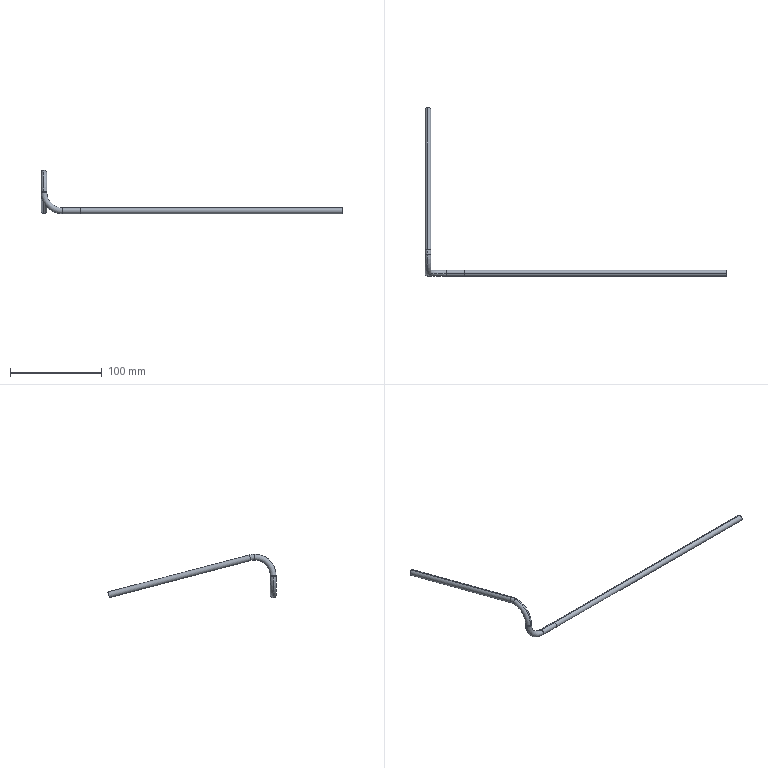Part | STEP file | copper tube 33_default_machined_ | 2 solids | 20 faces | box 328.675 x 183.099 x 47.35 mm | volume 11843 mm3 | cylinder 10 | torus 6 | plane 4 | commonest cylinder face diameters 6.35 x8 4.75 x2
STEP:
#1=CARTESIAN_POINT('',(0.,0.,0.));
#2=DIRECTION('',(0.,0.,1.));
#3=DIRECTION('',(1.,0.,0.));
#4=AXIS2_PLACEMENT_3D('',#1,#2,#3);
#5=CARTESIAN_POINT('',(285.5,0.,3.175));
#6=VERTEX_POINT('',#5);
#7=CARTESIAN_POINT('',(285.5,0.,-3.175));
#8=VERTEX_POINT('',#7);
#9=CARTESIAN_POINT('',(285.5,0.,0.));
#10=DIRECTION('',(-1.,0.,0.));
#11=DIRECTION('',(0.,0.,1.));
#12=AXIS2_PLACEMENT_3D('',#9,#10,#11);
#13=CIRCLE('',#12,3.175);
#14=CARTESIAN_POINT('',(285.5,0.,0.));
#15=DIRECTION('',(-1.,0.,0.));
#16=DIRECTION('',(0.,0.,1.));
#17=AXIS2_PLACEMENT_3D('',#14,#15,#16);
#18=CYLINDRICAL_SURFACE('',#17,3.175);
#19=CARTESIAN_POINT('',(0.,0.));
#20=DIRECTION('',(1.,0.));
#21=VECTOR('',#20,1.);
#22=LINE('',#19,#21);
#23=(GEOMETRIC_REPRESENTATION_CONTEXT(2)PARAMETRIC_REPRESENTATION_CONTEXT()REPRESENTATION_CONTEXT('',''));
#24=DEFINITIONAL_REPRESENTATION('',(#22),#23);
#25=PCURVE('',#18,#24);
#26=CARTESIAN_POINT('',(285.5,0.,0.));
#27=DIRECTION('',(1.,0.,0.));
#28=DIRECTION('',(0.,0.,-1.));
#29=AXIS2_PLACEMENT_3D('',#26,#27,#28);
#30=PLANE('',#29);
#31=CARTESIAN_POINT('',(-3.175,0.));
#32=CARTESIAN_POINT('',(-3.175,5.499));
#33=CARTESIAN_POINT('',(1.587,2.75));
#34=CARTESIAN_POINT('',(6.35,0.));
#35=CARTESIAN_POINT('',(1.587,-2.75));
#36=CARTESIAN_POINT('',(-3.175,-5.499));
#37=CARTESIAN_POINT('',(-3.175,0.));
#38=(BOUNDED_CURVE()B_SPLINE_CURVE(2,(#31,#32,#33,#34,#35,#36,#37),.UNSPECIFIED.,.T.,.F.)B_SPLINE_CURVE_WITH_KNOTS((1,2,2,2,2,1),(-2.094,0.,2.094,4.189,6.283,8.378),.UNSPECIFIED.)CURVE()GEOMETRIC_REPRESENTATION_ITEM()RATIONAL_B_SPLINE_CURVE((1.,0.5,1.,0.5,1.,0.5,1.))REPRESENTATION_ITEM(''));
#39=(GEOMETRIC_REPRESENTATION_CONTEXT(2)PARAMETRIC_REPRESENTATION_CONTEXT()REPRESENTATION_CONTEXT('',''));
#40=DEFINITIONAL_REPRESENTATION('',(#38),#39);
#41=PCURVE('',#30,#40);
#42=SURFACE_CURVE('',#13,(#25,#41),.PCURVE_S1.);
#43=EDGE_CURVE('',#6,#8,#42,.T.);
#44=ORIENTED_EDGE('',*,*,#43,.T.);
#45=CARTESIAN_POINT('',(0.,0.,-3.175));
#46=VERTEX_POINT('',#45);
#47=CARTESIAN_POINT('',(285.5,0.,-3.175));
#48=DIRECTION('',(-1.,0.,0.));
#49=VECTOR('',#48,1.);
#50=LINE('',#47,#49);
#51=CARTESIAN_POINT('',(3.142,0.));
#52=DIRECTION('',(0.,1.));
#53=VECTOR('',#52,1.);
#54=LINE('',#51,#53);
#55=(GEOMETRIC_REPRESENTATION_CONTEXT(2)PARAMETRIC_REPRESENTATION_CONTEXT()REPRESENTATION_CONTEXT('',''));
#56=DEFINITIONAL_REPRESENTATION('',(#54),#55);
#57=PCURVE('',#18,#56);
#58=CARTESIAN_POINT('',(285.5,0.,0.));
#59=DIRECTION('',(-1.,0.,0.));
#60=DIRECTION('',(0.,0.,1.));
#61=AXIS2_PLACEMENT_3D('',#58,#59,#60);
#62=CYLINDRICAL_SURFACE('',#61,3.175);
#63=CARTESIAN_POINT('',(3.142,0.));
#64=DIRECTION('',(0.,1.));
#65=VECTOR('',#64,1.);
#66=LINE('',#63,#65);
#67=(GEOMETRIC_REPRESENTATION_CONTEXT(2)PARAMETRIC_REPRESENTATION_CONTEXT()REPRESENTATION_CONTEXT('',''));
#68=DEFINITIONAL_REPRESENTATION('',(#66),#67);
#69=PCURVE('',#62,#68);
#70=SURFACE_CURVE('',#50,(#57,#69),.PCURVE_S1.);
#71=EDGE_CURVE('',#8,#46,#70,.T.);
#72=ORIENTED_EDGE('',*,*,#71,.T.);
#73=CARTESIAN_POINT('',(0.,0.,3.175));
#74=VERTEX_POINT('',#73);
#75=CARTESIAN_POINT('',(0.,0.,0.));
#76=DIRECTION('',(1.,0.,0.));
#77=DIRECTION('',(0.,0.,1.));
#78=AXIS2_PLACEMENT_3D('',#75,#76,#77);
#79=CIRCLE('',#78,3.175);
#80=CARTESIAN_POINT('',(6.283,285.5));
#81=DIRECTION('',(-1.,0.));
#82=VECTOR('',#81,1.);
#83=LINE('',#80,#82);
#84=(GEOMETRIC_REPRESENTATION_CONTEXT(2)PARAMETRIC_REPRESENTATION_CONTEXT()REPRESENTATION_CONTEXT('',''));
#85=DEFINITIONAL_REPRESENTATION('',(#83),#84);
#86=PCURVE('',#18,#85);
#87=CARTESIAN_POINT('',(0.,0.,0.));
#88=DIRECTION('',(1.,0.,0.));
#89=DIRECTION('',(0.,0.,-1.));
#90=AXIS2_PLACEMENT_3D('',#87,#88,#89);
#91=PLANE('',#90);
#92=CARTESIAN_POINT('',(0.,0.));
#93=DIRECTION('',(-1.,0.));
#94=AXIS2_PLACEMENT_2D('',#92,#93);
#95=CIRCLE('',#94,3.175);
#96=(GEOMETRIC_REPRESENTATION_CONTEXT(2)PARAMETRIC_REPRESENTATION_CONTEXT()REPRESENTATION_CONTEXT('',''));
#97=DEFINITIONAL_REPRESENTATION('',(#95),#96);
#98=PCURVE('',#91,#97);
#99=SURFACE_CURVE('',#79,(#86,#98),.PCURVE_S1.);
#100=EDGE_CURVE('',#46,#74,#99,.T.);
#101=ORIENTED_EDGE('',*,*,#100,.T.);
#102=CARTESIAN_POINT('',(285.5,0.,3.175));
#103=DIRECTION('',(-1.,0.,0.));
#104=VECTOR('',#103,1.);
#105=LINE('',#102,#104);
#106=CARTESIAN_POINT('',(0.,0.));
#107=DIRECTION('',(0.,1.));
#108=VECTOR('',#107,1.);
#109=LINE('',#106,#108);
#110=(GEOMETRIC_REPRESENTATION_CONTEXT(2)PARAMETRIC_REPRESENTATION_CONTEXT()REPRESENTATION_CONTEXT('',''));
#111=DEFINITIONAL_REPRESENTATION('',(#109),#110);
#112=PCURVE('',#18,#111);
#113=CARTESIAN_POINT('',(6.283,0.));
#114=DIRECTION('',(0.,1.));
#115=VECTOR('',#114,1.);
#116=LINE('',#113,#115);
#117=(GEOMETRIC_REPRESENTATION_CONTEXT(2)PARAMETRIC_REPRESENTATION_CONTEXT()REPRESENTATION_CONTEXT('',''));
#118=DEFINITIONAL_REPRESENTATION('',(#116),#117);
#119=PCURVE('',#62,#118);
#120=SURFACE_CURVE('',#105,(#112,#119),.PCURVE_S1.);
#121=EDGE_CURVE('',#6,#74,#120,.T.);
#122=ORIENTED_EDGE('',*,*,#121,.F.);
#123=EDGE_LOOP('',(#44,#72,#101,#122));
#124=FACE_BOUND('',#123,.T.);
#125=ADVANCED_FACE('',(#124),#18,.T.);
#126=CARTESIAN_POINT('',(285.5,0.,2.375));
#127=VERTEX_POINT('',#126);
#128=CARTESIAN_POINT('',(0.,0.,2.375));
#129=VERTEX_POINT('',#128);
#130=CARTESIAN_POINT('',(285.5,0.,2.375));
#131=DIRECTION('',(-1.,0.,0.));
#132=VECTOR('',#131,1.);
#133=LINE('',#130,#132);
#134=CARTESIAN_POINT('',(285.5,0.,0.));
#135=DIRECTION('',(-1.,0.,0.));
#136=DIRECTION('',(0.,0.,1.));
#137=AXIS2_PLACEMENT_3D('',#134,#135,#136);
#138=CYLINDRICAL_SURFACE('',#137,2.375);
#139=CARTESIAN_POINT('',(6.283,0.));
#140=DIRECTION('',(0.,1.));
#141=VECTOR('',#140,1.);
#142=LINE('',#139,#141);
#143=(GEOMETRIC_REPRESENTATION_CONTEXT(2)PARAMETRIC_REPRESENTATION_CONTEXT()REPRESENTATION_CONTEXT('',''));
#144=DEFINITIONAL_REPRESENTATION('',(#142),#143);
#145=PCURVE('',#138,#144);
#146=CARTESIAN_POINT('',(285.5,0.,0.));
#147=DIRECTION('',(-1.,0.,0.));
#148=DIRECTION('',(0.,0.,1.));
#149=AXIS2_PLACEMENT_3D('',#146,#147,#148);
#150=CYLINDRICAL_SURFACE('',#149,2.375);
#151=CARTESIAN_POINT('',(0.,0.));
#152=DIRECTION('',(0.,1.));
#153=VECTOR('',#152,1.);
#154=LINE('',#151,#153);
#155=(GEOMETRIC_REPRESENTATION_CONTEXT(2)PARAMETRIC_REPRESENTATION_CONTEXT()REPRESENTATION_CONTEXT('',''));
#156=DEFINITIONAL_REPRESENTATION('',(#154),#155);
#157=PCURVE('',#150,#156);
#158=SURFACE_CURVE('',#133,(#145,#157),.PCURVE_S1.);
#159=EDGE_CURVE('',#127,#129,#158,.T.);
#160=ORIENTED_EDGE('',*,*,#159,.T.);
#161=CARTESIAN_POINT('',(0.,0.,-2.375));
#162=VERTEX_POINT('',#161);
#163=CARTESIAN_POINT('',(0.,0.,0.));
#164=DIRECTION('',(-1.,0.,0.));
#165=DIRECTION('',(0.,0.,1.));
#166=AXIS2_PLACEMENT_3D('',#163,#164,#165);
#167=CIRCLE('',#166,2.375);
#168=CARTESIAN_POINT('',(0.,285.5));
#169=DIRECTION('',(1.,0.));
#170=VECTOR('',#169,1.);
#171=LINE('',#168,#170);
#172=(GEOMETRIC_REPRESENTATION_CONTEXT(2)PARAMETRIC_REPRESENTATION_CONTEXT()REPRESENTATION_CONTEXT('',''));
#173=DEFINITIONAL_REPRESENTATION('',(#171),#172);
#174=PCURVE('',#138,#173);
#175=CARTESIAN_POINT('',(-2.375,0.));
#176=CARTESIAN_POINT('',(-2.375,4.114));
#177=CARTESIAN_POINT('',(1.188,2.057));
#178=CARTESIAN_POINT('',(4.75,0.));
#179=CARTESIAN_POINT('',(1.188,-2.057));
#180=CARTESIAN_POINT('',(-2.375,-4.114));
#181=CARTESIAN_POINT('',(-2.375,0.));
#182=(BOUNDED_CURVE()B_SPLINE_CURVE(2,(#175,#176,#177,#178,#179,#180,#181),.UNSPECIFIED.,.T.,.F.)B_SPLINE_CURVE_WITH_KNOTS((1,2,2,2,2,1),(-2.094,0.,2.094,4.189,6.283,8.378),.UNSPECIFIED.)CURVE()GEOMETRIC_REPRESENTATION_ITEM()RATIONAL_B_SPLINE_CURVE((1.,0.5,1.,0.5,1.,0.5,1.))REPRESENTATION_ITEM(''));
#183=(GEOMETRIC_REPRESENTATION_CONTEXT(2)PARAMETRIC_REPRESENTATION_CONTEXT()REPRESENTATION_CONTEXT('',''));
#184=DEFINITIONAL_REPRESENTATION('',(#182),#183);
#185=PCURVE('',#91,#184);
#186=SURFACE_CURVE('',#167,(#174,#185),.PCURVE_S1.);
#187=EDGE_CURVE('',#162,#129,#186,.T.);
#188=ORIENTED_EDGE('',*,*,#187,.F.);
#189=CARTESIAN_POINT('',(285.5,0.,-2.375));
#190=VERTEX_POINT('',#189);
#191=CARTESIAN_POINT('',(285.5,0.,-2.375));
#192=DIRECTION('',(-1.,0.,0.));
#193=VECTOR('',#192,1.);
#194=LINE('',#191,#193);
#195=CARTESIAN_POINT('',(3.142,0.));
#196=DIRECTION('',(0.,1.));
#197=VECTOR('',#196,1.);
#198=LINE('',#195,#197);
#199=(GEOMETRIC_REPRESENTATION_CONTEXT(2)PARAMETRIC_REPRESENTATION_CONTEXT()REPRESENTATION_CONTEXT('',''));
#200=DEFINITIONAL_REPRESENTATION('',(#198),#199);
#201=PCURVE('',#138,#200);
#202=CARTESIAN_POINT('',(3.142,0.));
#203=DIRECTION('',(0.,1.));
#204=VECTOR('',#203,1.);
#205=LINE('',#202,#204);
#206=(GEOMETRIC_REPRESENTATION_CONTEXT(2)PARAMETRIC_REPRESENTATION_CONTEXT()REPRESENTATION_CONTEXT('',''));
#207=DEFINITIONAL_REPRESENTATION('',(#205),#206);
#208=PCURVE('',#150,#207);
#209=SURFACE_CURVE('',#194,(#201,#208),.PCURVE_S1.);
#210=EDGE_CURVE('',#190,#162,#209,.T.);
#211=ORIENTED_EDGE('',*,*,#210,.F.);
#212=CARTESIAN_POINT('',(285.5,0.,0.));
#213=DIRECTION('',(-1.,0.,0.));
#214=DIRECTION('',(0.,0.,1.));
#215=AXIS2_PLACEMENT_3D('',#212,#213,#214);
#216=CIRCLE('',#215,2.375);
#217=CARTESIAN_POINT('',(0.,0.));
#218=DIRECTION('',(1.,0.));
#219=VECTOR('',#218,1.);
#220=LINE('',#217,#219);
#221=(GEOMETRIC_REPRESENTATION_CONTEXT(2)PARAMETRIC_REPRESENTATION_CONTEXT()REPRESENTATION_CONTEXT('',''));
#222=DEFINITIONAL_REPRESENTATION('',(#220),#221);
#223=PCURVE('',#138,#222);
#224=CARTESIAN_POINT('',(-2.375,0.));
#225=CARTESIAN_POINT('',(-2.375,4.114));
#226=CARTESIAN_POINT('',(1.188,2.057));
#227=CARTESIAN_POINT('',(4.75,0.));
#228=CARTESIAN_POINT('',(1.188,-2.057));
#229=CARTESIAN_POINT('',(-2.375,-4.114));
#230=CARTESIAN_POINT('',(-2.375,0.));
#231=(BOUNDED_CURVE()B_SPLINE_CURVE(2,(#224,#225,#226,#227,#228,#229,#230),.UNSPECIFIED.,.T.,.F.)B_SPLINE_CURVE_WITH_KNOTS((1,2,2,2,2,1),(-2.094,0.,2.094,4.189,6.283,8.378),.UNSPECIFIED.)CURVE()GEOMETRIC_REPRESENTATION_ITEM()RATIONAL_B_SPLINE_CURVE((1.,0.5,1.,0.5,1.,0.5,1.))REPRESENTATION_ITEM(''));
#232=(GEOMETRIC_REPRESENTATION_CONTEXT(2)PARAMETRIC_REPRESENTATION_CONTEXT()REPRESENTATION_CONTEXT('',''));
#233=DEFINITIONAL_REPRESENTATION('',(#231),#232);
#234=PCURVE('',#30,#233);
#235=SURFACE_CURVE('',#216,(#223,#234),.PCURVE_S1.);
#236=EDGE_CURVE('',#190,#127,#235,.T.);
#237=ORIENTED_EDGE('',*,*,#236,.T.);
#238=EDGE_LOOP('',(#160,#188,#211,#237));
#239=FACE_BOUND('',#238,.F.);
#240=ADVANCED_FACE('',(#239),#138,.F.);
#241=ORIENTED_EDGE('',*,*,#71,.F.);
#242=CARTESIAN_POINT('',(285.5,0.,0.));
#243=DIRECTION('',(-1.,0.,0.));
#244=DIRECTION('',(0.,0.,1.));
#245=AXIS2_PLACEMENT_3D('',#242,#243,#244);
#246=CIRCLE('',#245,3.175);
#247=CARTESIAN_POINT('',(0.,0.));
#248=DIRECTION('',(1.,0.));
#249=VECTOR('',#248,1.);
#250=LINE('',#247,#249);
#251=(GEOMETRIC_REPRESENTATION_CONTEXT(2)PARAMETRIC_REPRESENTATION_CONTEXT()REPRESENTATION_CONTEXT('',''));
#252=DEFINITIONAL_REPRESENTATION('',(#250),#251);
#253=PCURVE('',#62,#252);
#254=CARTESIAN_POINT('',(-3.175,0.));
#255=CARTESIAN_POINT('',(-3.175,5.499));
#256=CARTESIAN_POINT('',(1.587,2.75));
#257=CARTESIAN_POINT('',(6.35,0.));
#258=CARTESIAN_POINT('',(1.587,-2.75));
#259=CARTESIAN_POINT('',(-3.175,-5.499));
#260=CARTESIAN_POINT('',(-3.175,0.));
#261=(BOUNDED_CURVE()B_SPLINE_CURVE(2,(#254,#255,#256,#257,#258,#259,#260),.UNSPECIFIED.,.T.,.F.)B_SPLINE_CURVE_WITH_KNOTS((1,2,2,2,2,1),(-2.094,0.,2.094,4.189,6.283,8.378),.UNSPECIFIED.)CURVE()GEOMETRIC_REPRESENTATION_ITEM()RATIONAL_B_SPLINE_CURVE((1.,0.5,1.,0.5,1.,0.5,1.))REPRESENTATION_ITEM(''));
#262=(GEOMETRIC_REPRESENTATION_CONTEXT(2)PARAMETRIC_REPRESENTATION_CONTEXT()REPRESENTATION_CONTEXT('',''));
#263=DEFINITIONAL_REPRESENTATION('',(#261),#262);
#264=PCURVE('',#30,#263);
#265=SURFACE_CURVE('',#246,(#253,#264),.PCURVE_S1.);
#266=EDGE_CURVE('',#8,#6,#265,.T.);
#267=ORIENTED_EDGE('',*,*,#266,.T.);
#268=ORIENTED_EDGE('',*,*,#121,.T.);
#269=CARTESIAN_POINT('',(0.,0.,0.));
#270=DIRECTION('',(1.,0.,0.));
#271=DIRECTION('',(0.,0.,1.));
#272=AXIS2_PLACEMENT_3D('',#269,#270,#271);
#273=CIRCLE('',#272,3.175);
#274=CARTESIAN_POINT('',(6.283,285.5));
#275=DIRECTION('',(-1.,0.));
#276=VECTOR('',#275,1.);
#277=LINE('',#274,#276);
#278=(GEOMETRIC_REPRESENTATION_CONTEXT(2)PARAMETRIC_REPRESENTATION_CONTEXT()REPRESENTATION_CONTEXT('',''));
#279=DEFINITIONAL_REPRESENTATION('',(#277),#278);
#280=PCURVE('',#62,#279);
#281=CARTESIAN_POINT('',(0.,0.));
#282=DIRECTION('',(-1.,0.));
#283=AXIS2_PLACEMENT_2D('',#281,#282);
#284=CIRCLE('',#283,3.175);
#285=(GEOMETRIC_REPRESENTATION_CONTEXT(2)PARAMETRIC_REPRESENTATION_CONTEXT()REPRESENTATION_CONTEXT('',''));
#286=DEFINITIONAL_REPRESENTATION('',(#284),#285);
#287=PCURVE('',#91,#286);
#288=SURFACE_CURVE('',#273,(#280,#287),.PCURVE_S1.);
#289=EDGE_CURVE('',#74,#46,#288,.T.);
#290=ORIENTED_EDGE('',*,*,#289,.T.);
#291=EDGE_LOOP('',(#241,#267,#268,#290));
#292=FACE_BOUND('',#291,.T.);
#293=ADVANCED_FACE('',(#292),#62,.T.);
#294=ORIENTED_EDGE('',*,*,#289,.F.);
#295=ORIENTED_EDGE('',*,*,#100,.F.);
#296=EDGE_LOOP('',(#294,#295));
#297=FACE_BOUND('',#296,.T.);
#298=CARTESIAN_POINT('',(0.,0.,0.));
#299=DIRECTION('',(-1.,0.,0.));
#300=DIRECTION('',(0.,0.,1.));
#301=AXIS2_PLACEMENT_3D('',#298,#299,#300);
#302=CIRCLE('',#301,2.375);
#303=CARTESIAN_POINT('',(-2.375,0.));
#304=CARTESIAN_POINT('',(-2.375,4.114));
#305=CARTESIAN_POINT('',(1.188,2.057));
#306=CARTESIAN_POINT('',(4.75,0.));
#307=CARTESIAN_POINT('',(1.188,-2.057));
#308=CARTESIAN_POINT('',(-2.375,-4.114));
#309=CARTESIAN_POINT('',(-2.375,0.));
#310=(BOUNDED_CURVE()B_SPLINE_CURVE(2,(#303,#304,#305,#306,#307,#308,#309),.UNSPECIFIED.,.T.,.F.)B_SPLINE_CURVE_WITH_KNOTS((1,2,2,2,2,1),(-2.094,0.,2.094,4.189,6.283,8.378),.UNSPECIFIED.)CURVE()GEOMETRIC_REPRESENTATION_ITEM()RATIONAL_B_SPLINE_CURVE((1.,0.5,1.,0.5,1.,0.5,1.))REPRESENTATION_ITEM(''));
#311=(GEOMETRIC_REPRESENTATION_CONTEXT(2)PARAMETRIC_REPRESENTATION_CONTEXT()REPRESENTATION_CONTEXT('',''));
#312=DEFINITIONAL_REPRESENTATION('',(#310),#311);
#313=PCURVE('',#91,#312);
#314=CARTESIAN_POINT('',(0.,285.5));
#315=DIRECTION('',(1.,0.));
#316=VECTOR('',#315,1.);
#317=LINE('',#314,#316);
#318=(GEOMETRIC_REPRESENTATION_CONTEXT(2)PARAMETRIC_REPRESENTATION_CONTEXT()REPRESENTATION_CONTEXT('',''));
#319=DEFINITIONAL_REPRESENTATION('',(#317),#318);
#320=PCURVE('',#150,#319);
#321=SURFACE_CURVE('',#302,(#313,#320),.PCURVE_S1.);
#322=EDGE_CURVE('',#129,#162,#321,.T.);
#323=ORIENTED_EDGE('',*,*,#322,.F.);
#324=ORIENTED_EDGE('',*,*,#187,.F.);
#325=EDGE_LOOP('',(#323,#324));
#326=FACE_BOUND('',#325,.T.);
#327=ADVANCED_FACE('',(#297,#326),#91,.F.);
#328=ORIENTED_EDGE('',*,*,#43,.F.);
#329=ORIENTED_EDGE('',*,*,#266,.F.);
#330=EDGE_LOOP('',(#328,#329));
#331=FACE_BOUND('',#330,.T.);
#332=CARTESIAN_POINT('',(285.5,0.,0.));
#333=DIRECTION('',(-1.,0.,0.));
#334=DIRECTION('',(0.,0.,1.));
#335=AXIS2_PLACEMENT_3D('',#332,#333,#334);
#336=CIRCLE('',#335,2.375);
#337=CARTESIAN_POINT('',(-2.375,0.));
#338=CARTESIAN_POINT('',(-2.375,4.114));
#339=CARTESIAN_POINT('',(1.188,2.057));
#340=CARTESIAN_POINT('',(4.75,0.));
#341=CARTESIAN_POINT('',(1.188,-2.057));
#342=CARTESIAN_POINT('',(-2.375,-4.114));
#343=CARTESIAN_POINT('',(-2.375,0.));
#344=(BOUNDED_CURVE()B_SPLINE_CURVE(2,(#337,#338,#339,#340,#341,#342,#343),.UNSPECIFIED.,.T.,.F.)B_SPLINE_CURVE_WITH_KNOTS((1,2,2,2,2,1),(-2.094,0.,2.094,4.189,6.283,8.378),.UNSPECIFIED.)CURVE()GEOMETRIC_REPRESENTATION_ITEM()RATIONAL_B_SPLINE_CURVE((1.,0.5,1.,0.5,1.,0.5,1.))REPRESENTATION_ITEM(''));
#345=(GEOMETRIC_REPRESENTATION_CONTEXT(2)PARAMETRIC_REPRESENTATION_CONTEXT()REPRESENTATION_CONTEXT('',''));
#346=DEFINITIONAL_REPRESENTATION('',(#344),#345);
#347=PCURVE('',#30,#346);
#348=CARTESIAN_POINT('',(0.,0.));
#349=DIRECTION('',(1.,0.));
#350=VECTOR('',#349,1.);
#351=LINE('',#348,#350);
#352=(GEOMETRIC_REPRESENTATION_CONTEXT(2)PARAMETRIC_REPRESENTATION_CONTEXT()REPRESENTATION_CONTEXT('',''));
#353=DEFINITIONAL_REPRESENTATION('',(#351),#352);
#354=PCURVE('',#150,#353);
#355=SURFACE_CURVE('',#336,(#347,#354),.PCURVE_S1.);
#356=EDGE_CURVE('',#127,#190,#355,.T.);
#357=ORIENTED_EDGE('',*,*,#356,.T.);
#358=ORIENTED_EDGE('',*,*,#236,.T.);
#359=EDGE_LOOP('',(#357,#358));
#360=FACE_BOUND('',#359,.T.);
#361=ADVANCED_FACE('',(#331,#360),#30,.T.);
#362=ORIENTED_EDGE('',*,*,#322,.F.);
#363=ORIENTED_EDGE('',*,*,#159,.F.);
#364=ORIENTED_EDGE('',*,*,#356,.T.);
#365=ORIENTED_EDGE('',*,*,#210,.T.);
#366=EDGE_LOOP('',(#362,#363,#364,#365));
#367=FACE_BOUND('',#366,.F.);
#368=ADVANCED_FACE('',(#367),#150,.F.);
#369=CLOSED_SHELL('',(#125,#240,#293,#327,#361,#368));
#370=MANIFOLD_SOLID_BREP('',#369);
#371=CARTESIAN_POINT('',(-20.,0.,3.175));
#372=VERTEX_POINT('',#371);
#373=CARTESIAN_POINT('',(-20.,0.,-3.175));
#374=VERTEX_POINT('',#373);
#375=CARTESIAN_POINT('',(-20.,0.,0.));
#376=DIRECTION('',(-1.,0.,0.));
#377=DIRECTION('',(0.,0.,1.));
#378=AXIS2_PLACEMENT_3D('',#375,#376,#377);
#379=CIRCLE('',#378,3.175);
#380=CARTESIAN_POINT('',(-20.,0.,20.));
#381=DIRECTION('',(0.,1.,0.));
#382=DIRECTION('',(0.,0.,1.));
#383=AXIS2_PLACEMENT_3D('',#380,#381,#382);
#384=TOROIDAL_SURFACE('',#383,20.,3.175);
#385=CARTESIAN_POINT('',(3.142,3.142));
#386=DIRECTION('',(0.,-1.));
#387=VECTOR('',#386,1.);
#388=LINE('',#385,#387);
#389=(GEOMETRIC_REPRESENTATION_CONTEXT(2)PARAMETRIC_REPRESENTATION_CONTEXT()REPRESENTATION_CONTEXT('',''));
#390=DEFINITIONAL_REPRESENTATION('',(#388),#389);
#391=PCURVE('',#384,#390);
#392=CARTESIAN_POINT('',(-20.,0.,0.));
#393=DIRECTION('',(1.,0.,0.));
#394=DIRECTION('',(0.,0.,-1.));
#395=AXIS2_PLACEMENT_3D('',#392,#393,#394);
#396=CYLINDRICAL_SURFACE('',#395,3.175);
#397=CARTESIAN_POINT('',(3.142,0.));
#398=DIRECTION('',(-1.,0.));
#399=VECTOR('',#398,1.);
#400=LINE('',#397,#399);
#401=(GEOMETRIC_REPRESENTATION_CONTEXT(2)PARAMETRIC_REPRESENTATION_CONTEXT()REPRESENTATION_CONTEXT('',''));
#402=DEFINITIONAL_REPRESENTATION('',(#400),#401);
#403=PCURVE('',#396,#402);
#404=SURFACE_CURVE('',#379,(#391,#403),.PCURVE_S1.);
#405=EDGE_CURVE('',#372,#374,#404,.T.);
#406=ORIENTED_EDGE('',*,*,#405,.T.);
#407=CARTESIAN_POINT('',(-43.175,0.,20.));
#408=VERTEX_POINT('',#407);
#409=CARTESIAN_POINT('',(-20.,0.,20.));
#410=DIRECTION('',(0.,1.,0.));
#411=DIRECTION('',(0.,0.,1.));
#412=AXIS2_PLACEMENT_3D('',#409,#410,#411);
#413=CIRCLE('',#412,23.175);
#414=CARTESIAN_POINT('',(0.,0.));
#415=DIRECTION('',(1.,0.));
#416=VECTOR('',#415,1.);
#417=LINE('',#414,#416);
#418=(GEOMETRIC_REPRESENTATION_CONTEXT(2)PARAMETRIC_REPRESENTATION_CONTEXT()REPRESENTATION_CONTEXT('',''));
#419=DEFINITIONAL_REPRESENTATION('',(#417),#418);
#420=PCURVE('',#384,#419);
#421=CARTESIAN_POINT('',(-20.,0.,20.));
#422=DIRECTION('',(0.,1.,0.));
#423=DIRECTION('',(0.,0.,1.));
#424=AXIS2_PLACEMENT_3D('',#421,#422,#423);
#425=TOROIDAL_SURFACE('',#424,20.,3.175);
#426=CARTESIAN_POINT('',(0.,6.283));
#427=DIRECTION('',(1.,0.));
#428=VECTOR('',#427,1.);
#429=LINE('',#426,#428);
#430=(GEOMETRIC_REPRESENTATION_CONTEXT(2)PARAMETRIC_REPRESENTATION_CONTEXT()REPRESENTATION_CONTEXT('',''));
#431=DEFINITIONAL_REPRESENTATION('',(#429),#430);
#432=PCURVE('',#425,#431);
#433=SURFACE_CURVE('',#413,(#420,#432),.PCURVE_S1.);
#434=EDGE_CURVE('',#374,#408,#433,.T.);
#435=ORIENTED_EDGE('',*,*,#434,.T.);
#436=CARTESIAN_POINT('',(-40.,3.175,20.));
#437=VERTEX_POINT('',#436);
#438=CARTESIAN_POINT('',(-40.,0.,20.));
#439=DIRECTION('',(0.,0.,1.));
#440=DIRECTION('',(1.,0.,0.));
#441=AXIS2_PLACEMENT_3D('',#438,#439,#440);
#442=CIRCLE('',#441,3.175);
#443=CARTESIAN_POINT('',(4.712,3.142));
#444=DIRECTION('',(0.,-1.));
#445=VECTOR('',#444,1.);
#446=LINE('',#443,#445);
#447=(GEOMETRIC_REPRESENTATION_CONTEXT(2)PARAMETRIC_REPRESENTATION_CONTEXT()REPRESENTATION_CONTEXT('',''));
#448=DEFINITIONAL_REPRESENTATION('',(#446),#447);
#449=PCURVE('',#384,#448);
#450=CARTESIAN_POINT('',(-40.,0.,20.));
#451=DIRECTION('',(0.,0.,1.));
#452=DIRECTION('',(0.,-1.,0.));
#453=AXIS2_PLACEMENT_3D('',#450,#451,#452);
#454=CYLINDRICAL_SURFACE('',#453,3.175);
#455=CARTESIAN_POINT('',(1.571,0.));
#456=DIRECTION('',(1.,0.));
#457=VECTOR('',#456,1.);
#458=LINE('',#455,#457);
#459=(GEOMETRIC_REPRESENTATION_CONTEXT(2)PARAMETRIC_REPRESENTATION_CONTEXT()REPRESENTATION_CONTEXT('',''));
#460=DEFINITIONAL_REPRESENTATION('',(#458),#459);
#461=PCURVE('',#454,#460);
#462=SURFACE_CURVE('',#442,(#449,#461),.PCURVE_S1.);
#463=EDGE_CURVE('',#437,#408,#462,.T.);
#464=ORIENTED_EDGE('',*,*,#463,.F.);
#465=CARTESIAN_POINT('',(-36.825,0.,20.));
#466=VERTEX_POINT('',#465);
#467=CARTESIAN_POINT('',(-40.,0.,20.));
#468=DIRECTION('',(0.,0.,1.));
#469=DIRECTION('',(1.,0.,0.));
#470=AXIS2_PLACEMENT_3D('',#467,#468,#469);
#471=CIRCLE('',#470,3.175);
#472=CARTESIAN_POINT('',(4.712,3.142));
#473=DIRECTION('',(0.,-1.));
#474=VECTOR('',#473,1.);
#475=LINE('',#472,#474);
#476=(GEOMETRIC_REPRESENTATION_CONTEXT(2)PARAMETRIC_REPRESENTATION_CONTEXT()REPRESENTATION_CONTEXT('',''));
#477=DEFINITIONAL_REPRESENTATION('',(#475),#476);
#478=PCURVE('',#384,#477);
#479=CARTESIAN_POINT('',(-40.,0.,20.));
#480=DIRECTION('',(0.,0.,1.));
#481=DIRECTION('',(0.,-1.,0.));
#482=AXIS2_PLACEMENT_3D('',#479,#480,#481);
#483=CYLINDRICAL_SURFACE('',#482,3.175);
#484=CARTESIAN_POINT('',(1.571,0.));
#485=DIRECTION('',(1.,0.));
#486=VECTOR('',#485,1.);
#487=LINE('',#484,#486);
#488=(GEOMETRIC_REPRESENTATION_CONTEXT(2)PARAMETRIC_REPRESENTATION_CONTEXT()REPRESENTATION_CONTEXT('',''));
#489=DEFINITIONAL_REPRESENTATION('',(#487),#488);
#490=PCURVE('',#483,#489);
#491=SURFACE_CURVE('',#471,(#478,#490),.PCURVE_S1.);
#492=EDGE_CURVE('',#466,#437,#491,.T.);
#493=ORIENTED_EDGE('',*,*,#492,.F.);
#494=CARTESIAN_POINT('',(-20.,0.,20.));
#495=DIRECTION('',(0.,1.,0.));
#496=DIRECTION('',(0.,0.,1.));
#497=AXIS2_PLACEMENT_3D('',#494,#495,#496);
#498=CIRCLE('',#497,16.825);
#499=CARTESIAN_POINT('',(0.,3.142));
#500=DIRECTION('',(1.,0.));
#501=VECTOR('',#500,1.);
#502=LINE('',#499,#501);
#503=(GEOMETRIC_REPRESENTATION_CONTEXT(2)PARAMETRIC_REPRESENTATION_CONTEXT()REPRESENTATION_CONTEXT('',''));
#504=DEFINITIONAL_REPRESENTATION('',(#502),#503);
#505=PCURVE('',#384,#504);
#506=CARTESIAN_POINT('',(0.,3.142));
#507=DIRECTION('',(1.,0.));
#508=VECTOR('',#507,1.);
#509=LINE('',#506,#508);
#510=(GEOMETRIC_REPRESENTATION_CONTEXT(2)PARAMETRIC_REPRESENTATION_CONTEXT()REPRESENTATION_CONTEXT('',''));
#511=DEFINITIONAL_REPRESENTATION('',(#509),#510);
#512=PCURVE('',#425,#511);
#513=SURFACE_CURVE('',#498,(#505,#512),.PCURVE_S1.);
#514=EDGE_CURVE('',#372,#466,#513,.T.);
#515=ORIENTED_EDGE('',*,*,#514,.F.);
#516=EDGE_LOOP('',(#406,#435,#464,#493,#515));
#517=FACE_BOUND('',#516,.T.);
#518=ADVANCED_FACE('',(#517),#384,.T.);
#519=CARTESIAN_POINT('',(-40.,20.,44.175));
#520=VERTEX_POINT('',#519);
#521=CARTESIAN_POINT('',(-40.,20.,37.825));
#522=VERTEX_POINT('',#521);
#523=CARTESIAN_POINT('',(-40.,20.,41.));
#524=DIRECTION('',(0.,-1.,0.));
#525=DIRECTION('',(0.,0.,-1.));
#526=AXIS2_PLACEMENT_3D('',#523,#524,#525);
#527=CIRCLE('',#526,3.175);
#528=CARTESIAN_POINT('',(-40.,20.,21.));
#529=DIRECTION('',(-1.,0.,0.));
#530=DIRECTION('',(0.,0.,1.));
#531=AXIS2_PLACEMENT_3D('',#528,#529,#530);
#532=TOROIDAL_SURFACE('',#531,20.,3.175);
#533=CARTESIAN_POINT('',(0.,-3.142));
#534=DIRECTION('',(0.,1.));
#535=VECTOR('',#534,1.);
#536=LINE('',#533,#535);
#537=(GEOMETRIC_REPRESENTATION_CONTEXT(2)PARAMETRIC_REPRESENTATION_CONTEXT()REPRESENTATION_CONTEXT('',''));
#538=DEFINITIONAL_REPRESENTATION('',(#536),#537);
#539=PCURVE('',#532,#538);
#540=CARTESIAN_POINT('',(-40.,20.,21.));
#541=DIRECTION('',(-1.,0.,0.));
#542=DIRECTION('',(0.,0.,1.));
#543=AXIS2_PLACEMENT_3D('',#540,#541,#542);
#544=TOROIDAL_SURFACE('',#543,20.,3.175);
#545=CARTESIAN_POINT('',(6.283,-3.142));
#546=DIRECTION('',(0.,1.));
#547=VECTOR('',#546,1.);
#548=LINE('',#545,#547);
#549=(GEOMETRIC_REPRESENTATION_CONTEXT(2)PARAMETRIC_REPRESENTATION_CONTEXT()REPRESENTATION_CONTEXT('',''));
#550=DEFINITIONAL_REPRESENTATION('',(#548),#549);
#551=PCURVE('',#544,#550);
#552=SURFACE_CURVE('',#527,(#539,#551),.PCURVE_S1.);
#553=EDGE_CURVE('',#520,#522,#552,.T.);
#554=ORIENTED_EDGE('',*,*,#553,.F.);
#555=CARTESIAN_POINT('',(-40.,25.872,43.419));
#556=VERTEX_POINT('',#555);
#557=CARTESIAN_POINT('',(-40.,20.,21.));
#558=DIRECTION('',(-1.,0.,0.));
#559=DIRECTION('',(0.,0.,1.));
#560=AXIS2_PLACEMENT_3D('',#557,#558,#559);
#561=CIRCLE('',#560,23.175);
#562=CARTESIAN_POINT('',(0.,0.));
#563=DIRECTION('',(1.,0.));
#564=VECTOR('',#563,1.);
#565=LINE('',#562,#564);
#566=(GEOMETRIC_REPRESENTATION_CONTEXT(2)PARAMETRIC_REPRESENTATION_CONTEXT()REPRESENTATION_CONTEXT('',''));
#567=DEFINITIONAL_REPRESENTATION('',(#565),#566);
#568=PCURVE('',#532,#567);
#569=CARTESIAN_POINT('',(-40.,20.,21.));
#570=DIRECTION('',(-1.,0.,0.));
#571=DIRECTION('',(0.,0.,1.));
#572=AXIS2_PLACEMENT_3D('',#569,#570,#571);
#573=TOROIDAL_SURFACE('',#572,20.,3.175);
#574=CARTESIAN_POINT('',(0.,6.283));
#575=DIRECTION('',(1.,0.));
#576=VECTOR('',#575,1.);
#577=LINE('',#574,#576);
#578=(GEOMETRIC_REPRESENTATION_CONTEXT(2)PARAMETRIC_REPRESENTATION_CONTEXT()REPRESENTATION_CONTEXT('',''));
#579=DEFINITIONAL_REPRESENTATION('',(#577),#578);
#580=PCURVE('',#573,#579);
#581=SURFACE_CURVE('',#561,(#568,#580),.PCURVE_S1.);
#582=EDGE_CURVE('',#520,#556,#581,.T.);
#583=ORIENTED_EDGE('',*,*,#582,.T.);
#584=CARTESIAN_POINT('',(-40.,24.263,37.276));
#585=VERTEX_POINT('',#584);
#586=CARTESIAN_POINT('',(-40.,25.067,40.347));
#587=DIRECTION('',(0.,0.9674,-0.2534));
#588=DIRECTION('',(1.,0.,0.));
#589=AXIS2_PLACEMENT_3D('',#586,#587,#588);
#590=CIRCLE('',#589,3.175);
#591=CARTESIAN_POINT('',(0.2562,4.712));
#592=DIRECTION('',(0.,-1.));
#593=VECTOR('',#592,1.);
#594=LINE('',#591,#593);
#595=(GEOMETRIC_REPRESENTATION_CONTEXT(2)PARAMETRIC_REPRESENTATION_CONTEXT()REPRESENTATION_CONTEXT('',''));
#596=DEFINITIONAL_REPRESENTATION('',(#594),#595);
#597=PCURVE('',#532,#596);
#598=CARTESIAN_POINT('',(-40.,25.067,40.347));
#599=DIRECTION('',(0.,0.9674,-0.2534));
#600=DIRECTION('',(0.,0.2534,0.9674));
#601=AXIS2_PLACEMENT_3D('',#598,#599,#600);
#602=CYLINDRICAL_SURFACE('',#601,3.175);
#603=CARTESIAN_POINT('',(1.571,0.));
#604=DIRECTION('',(1.,0.));
#605=VECTOR('',#604,1.);
#606=LINE('',#603,#605);
#607=(GEOMETRIC_REPRESENTATION_CONTEXT(2)PARAMETRIC_REPRESENTATION_CONTEXT()REPRESENTATION_CONTEXT('',''));
#608=DEFINITIONAL_REPRESENTATION('',(#606),#607);
#609=PCURVE('',#602,#608);
#610=SURFACE_CURVE('',#590,(#597,#609),.PCURVE_S1.);
#611=EDGE_CURVE('',#585,#556,#610,.T.);
#612=ORIENTED_EDGE('',*,*,#611,.F.);
#613=CARTESIAN_POINT('',(-40.,20.,21.));
#614=DIRECTION('',(-1.,0.,0.));
#615=DIRECTION('',(0.,0.,1.));
#616=AXIS2_PLACEMENT_3D('',#613,#614,#615);
#617=CIRCLE('',#616,16.825);
#618=CARTESIAN_POINT('',(0.,3.142));
#619=DIRECTION('',(1.,0.));
#620=VECTOR('',#619,1.);
#621=LINE('',#618,#620);
#622=(GEOMETRIC_REPRESENTATION_CONTEXT(2)PARAMETRIC_REPRESENTATION_CONTEXT()REPRESENTATION_CONTEXT('',''));
#623=DEFINITIONAL_REPRESENTATION('',(#621),#622);
#624=PCURVE('',#532,#623);
#625=CARTESIAN_POINT('',(0.,3.142));
#626=DIRECTION('',(1.,0.));
#627=VECTOR('',#626,1.);
#628=LINE('',#625,#627);
#629=(GEOMETRIC_REPRESENTATION_CONTEXT(2)PARAMETRIC_REPRESENTATION_CONTEXT()REPRESENTATION_CONTEXT('',''));
#630=DEFINITIONAL_REPRESENTATION('',(#628),#629);
#631=PCURVE('',#573,#630);
#632=SURFACE_CURVE('',#617,(#624,#631),.PCURVE_S1.);
#633=EDGE_CURVE('',#522,#585,#632,.T.);
#634=ORIENTED_EDGE('',*,*,#633,.F.);
#635=EDGE_LOOP('',(#554,#583,#612,#634));
#636=FACE_BOUND('',#635,.T.);
#637=ADVANCED_FACE('',(#636),#532,.T.);
#638=CARTESIAN_POINT('',(-40.,3.175,21.));
#639=VERTEX_POINT('',#638);
#640=CARTESIAN_POINT('',(-40.,-3.175,21.));
#641=VERTEX_POINT('',#640);
#642=CARTESIAN_POINT('',(-40.,0.,21.));
#643=DIRECTION('',(0.,0.,1.));
#644=DIRECTION('',(1.,0.,0.));
#645=AXIS2_PLACEMENT_3D('',#642,#643,#644);
#646=CIRCLE('',#645,3.175);
#647=CARTESIAN_POINT('',(4.712,4.712));
#648=DIRECTION('',(0.,-1.));
#649=VECTOR('',#648,1.);
#650=LINE('',#647,#649);
#651=(GEOMETRIC_REPRESENTATION_CONTEXT(2)PARAMETRIC_REPRESENTATION_CONTEXT()REPRESENTATION_CONTEXT('',''));
#652=DEFINITIONAL_REPRESENTATION('',(#650),#651);
#653=PCURVE('',#544,#652);
#654=CARTESIAN_POINT('',(1.571,1.));
#655=DIRECTION('',(1.,0.));
#656=VECTOR('',#655,1.);
#657=LINE('',#654,#656);
#658=(GEOMETRIC_REPRESENTATION_CONTEXT(2)PARAMETRIC_REPRESENTATION_CONTEXT()REPRESENTATION_CONTEXT('',''));
#659=DEFINITIONAL_REPRESENTATION('',(#657),#658);
#660=PCURVE('',#454,#659);
#661=SURFACE_CURVE('',#646,(#653,#660),.PCURVE_S1.);
#662=EDGE_CURVE('',#639,#641,#661,.T.);
#663=ORIENTED_EDGE('',*,*,#662,.T.);
#664=CARTESIAN_POINT('',(-40.,20.,21.));
#665=DIRECTION('',(-1.,0.,0.));
#666=DIRECTION('',(0.,0.,1.));
#667=AXIS2_PLACEMENT_3D('',#664,#665,#666);
#668=CIRCLE('',#667,23.175);
#669=CARTESIAN_POINT('',(0.,0.));
#670=DIRECTION('',(1.,0.));
#671=VECTOR('',#670,1.);
#672=LINE('',#669,#671);
#673=(GEOMETRIC_REPRESENTATION_CONTEXT(2)PARAMETRIC_REPRESENTATION_CONTEXT()REPRESENTATION_CONTEXT('',''));
#674=DEFINITIONAL_REPRESENTATION('',(#672),#673);
#675=PCURVE('',#544,#674);
#676=CARTESIAN_POINT('',(-40.,20.,21.));
#677=DIRECTION('',(-1.,0.,0.));
#678=DIRECTION('',(0.,0.,1.));
#679=AXIS2_PLACEMENT_3D('',#676,#677,#678);
#680=TOROIDAL_SURFACE('',#679,20.,3.175);
#681=CARTESIAN_POINT('',(0.,6.283));
#682=DIRECTION('',(1.,0.));
#683=VECTOR('',#682,1.);
#684=LINE('',#681,#683);
#685=(GEOMETRIC_REPRESENTATION_CONTEXT(2)PARAMETRIC_REPRESENTATION_CONTEXT()REPRESENTATION_CONTEXT('',''));
#686=DEFINITIONAL_REPRESENTATION('',(#684),#685);
#687=PCURVE('',#680,#686);
#688=SURFACE_CURVE('',#668,(#675,#687),.PCURVE_S1.);
#689=EDGE_CURVE('',#641,#520,#688,.T.);
#690=ORIENTED_EDGE('',*,*,#689,.T.);
#691=ORIENTED_EDGE('',*,*,#553,.T.);
#692=CARTESIAN_POINT('',(-40.,20.,21.));
#693=DIRECTION('',(-1.,0.,0.));
#694=DIRECTION('',(0.,0.,1.));
#695=AXIS2_PLACEMENT_3D('',#692,#693,#694);
#696=CIRCLE('',#695,16.825);
#697=CARTESIAN_POINT('',(0.,3.142));
#698=DIRECTION('',(1.,0.));
#699=VECTOR('',#698,1.);
#700=LINE('',#697,#699);
#701=(GEOMETRIC_REPRESENTATION_CONTEXT(2)PARAMETRIC_REPRESENTATION_CONTEXT()REPRESENTATION_CONTEXT('',''));
#702=DEFINITIONAL_REPRESENTATION('',(#700),#701);
#703=PCURVE('',#544,#702);
#704=CARTESIAN_POINT('',(0.,3.142));
#705=DIRECTION('',(1.,0.));
#706=VECTOR('',#705,1.);
#707=LINE('',#704,#706);
#708=(GEOMETRIC_REPRESENTATION_CONTEXT(2)PARAMETRIC_REPRESENTATION_CONTEXT()REPRESENTATION_CONTEXT('',''));
#709=DEFINITIONAL_REPRESENTATION('',(#707),#708);
#710=PCURVE('',#680,#709);
#711=SURFACE_CURVE('',#696,(#703,#710),.PCURVE_S1.);
#712=EDGE_CURVE('',#639,#522,#711,.T.);
#713=ORIENTED_EDGE('',*,*,#712,.F.);
#714=EDGE_LOOP('',(#663,#690,#691,#713));
#715=FACE_BOUND('',#714,.T.);
#716=ADVANCED_FACE('',(#715),#544,.T.);
#717=ORIENTED_EDGE('',*,*,#405,.F.);
#718=CARTESIAN_POINT('',(0.,0.,3.175));
#719=VERTEX_POINT('',#718);
#720=CARTESIAN_POINT('',(-20.,0.,3.175));
#721=DIRECTION('',(1.,0.,0.));
#722=VECTOR('',#721,1.);
#723=LINE('',#720,#722);
#724=CARTESIAN_POINT('',(3.142,0.));
#725=DIRECTION('',(0.,1.));
#726=VECTOR('',#725,1.);
#727=LINE('',#724,#726);
#728=(GEOMETRIC_REPRESENTATION_CONTEXT(2)PARAMETRIC_REPRESENTATION_CONTEXT()REPRESENTATION_CONTEXT('',''));
#729=DEFINITIONAL_REPRESENTATION('',(#727),#728);
#730=PCURVE('',#396,#729);
#731=CARTESIAN_POINT('',(-20.,0.,0.));
#732=DIRECTION('',(1.,0.,0.));
#733=DIRECTION('',(0.,0.,-1.));
#734=AXIS2_PLACEMENT_3D('',#731,#732,#733);
#735=CYLINDRICAL_SURFACE('',#734,3.175);
#736=CARTESIAN_POINT('',(3.142,0.));
#737=DIRECTION('',(0.,1.));
#738=VECTOR('',#737,1.);
#739=LINE('',#736,#738);
#740=(GEOMETRIC_REPRESENTATION_CONTEXT(2)PARAMETRIC_REPRESENTATION_CONTEXT()REPRESENTATION_CONTEXT('',''));
#741=DEFINITIONAL_REPRESENTATION('',(#739),#740);
#742=PCURVE('',#735,#741);
#743=SURFACE_CURVE('',#723,(#730,#742),.PCURVE_S1.);
#744=EDGE_CURVE('',#372,#719,#743,.T.);
#745=ORIENTED_EDGE('',*,*,#744,.T.);
#746=CARTESIAN_POINT('',(0.,0.,-3.175));
#747=VERTEX_POINT('',#746);
#748=CARTESIAN_POINT('',(0.,0.,0.));
#749=DIRECTION('',(-1.,0.,0.));
#750=DIRECTION('',(0.,0.,1.));
#751=AXIS2_PLACEMENT_3D('',#748,#749,#750);
#752=CIRCLE('',#751,3.175);
#753=CARTESIAN_POINT('',(3.142,20.));
#754=DIRECTION('',(-1.,0.));
#755=VECTOR('',#754,1.);
#756=LINE('',#753,#755);
#757=(GEOMETRIC_REPRESENTATION_CONTEXT(2)PARAMETRIC_REPRESENTATION_CONTEXT()REPRESENTATION_CONTEXT('',''));
#758=DEFINITIONAL_REPRESENTATION('',(#756),#757);
#759=PCURVE('',#396,#758);
#760=CARTESIAN_POINT('',(0.,0.,0.));
#761=DIRECTION('',(-1.,0.,0.));
#762=DIRECTION('',(0.,0.,1.));
#763=AXIS2_PLACEMENT_3D('',#760,#761,#762);
#764=PLANE('',#763);
#765=CARTESIAN_POINT('',(0.,0.));
#766=DIRECTION('',(1.,0.));
#767=AXIS2_PLACEMENT_2D('',#765,#766);
#768=CIRCLE('',#767,3.175);
#769=(GEOMETRIC_REPRESENTATION_CONTEXT(2)PARAMETRIC_REPRESENTATION_CONTEXT()REPRESENTATION_CONTEXT('',''));
#770=DEFINITIONAL_REPRESENTATION('',(#768),#769);
#771=PCURVE('',#764,#770);
#772=SURFACE_CURVE('',#752,(#759,#771),.PCURVE_S1.);
#773=EDGE_CURVE('',#719,#747,#772,.T.);
#774=ORIENTED_EDGE('',*,*,#773,.T.);
#775=CARTESIAN_POINT('',(-20.,0.,-3.175));
#776=DIRECTION('',(1.,0.,0.));
#777=VECTOR('',#776,1.);
#778=LINE('',#775,#777);
#779=CARTESIAN_POINT('',(0.,0.));
#780=DIRECTION('',(0.,1.));
#781=VECTOR('',#780,1.);
#782=LINE('',#779,#781);
#783=(GEOMETRIC_REPRESENTATION_CONTEXT(2)PARAMETRIC_REPRESENTATION_CONTEXT()REPRESENTATION_CONTEXT('',''));
#784=DEFINITIONAL_REPRESENTATION('',(#782),#783);
#785=PCURVE('',#396,#784);
#786=CARTESIAN_POINT('',(6.283,0.));
#787=DIRECTION('',(0.,1.));
#788=VECTOR('',#787,1.);
#789=LINE('',#786,#788);
#790=(GEOMETRIC_REPRESENTATION_CONTEXT(2)PARAMETRIC_REPRESENTATION_CONTEXT()REPRESENTATION_CONTEXT('',''));
#791=DEFINITIONAL_REPRESENTATION('',(#789),#790);
#792=PCURVE('',#735,#791);
#793=SURFACE_CURVE('',#778,(#785,#792),.PCURVE_S1.);
#794=EDGE_CURVE('',#374,#747,#793,.T.);
#795=ORIENTED_EDGE('',*,*,#794,.F.);
#796=EDGE_LOOP('',(#717,#745,#774,#795));
#797=FACE_BOUND('',#796,.T.);
#798=ADVANCED_FACE('',(#797),#396,.T.);
#799=CARTESIAN_POINT('',(-40.,-3.175,20.));
#800=VERTEX_POINT('',#799);
#801=CARTESIAN_POINT('',(-40.,0.,20.));
#802=DIRECTION('',(0.,0.,1.));
#803=DIRECTION('',(1.,0.,0.));
#804=AXIS2_PLACEMENT_3D('',#801,#802,#803);
#805=CIRCLE('',#804,3.175);
#806=CARTESIAN_POINT('',(-4.712,0.));
#807=DIRECTION('',(1.,0.));
#808=VECTOR('',#807,1.);
#809=LINE('',#806,#808);
#810=(GEOMETRIC_REPRESENTATION_CONTEXT(2)PARAMETRIC_REPRESENTATION_CONTEXT()REPRESENTATION_CONTEXT('',''));
#811=DEFINITIONAL_REPRESENTATION('',(#809),#810);
#812=PCURVE('',#483,#811);
#813=CARTESIAN_POINT('',(4.712,9.425));
#814=DIRECTION('',(0.,-1.));
#815=VECTOR('',#814,1.);
#816=LINE('',#813,#815);
#817=(GEOMETRIC_REPRESENTATION_CONTEXT(2)PARAMETRIC_REPRESENTATION_CONTEXT()REPRESENTATION_CONTEXT('',''));
#818=DEFINITIONAL_REPRESENTATION('',(#816),#817);
#819=PCURVE('',#425,#818);
#820=SURFACE_CURVE('',#805,(#812,#819),.PCURVE_S1.);
#821=EDGE_CURVE('',#800,#466,#820,.T.);
#822=ORIENTED_EDGE('',*,*,#821,.T.);
#823=ORIENTED_EDGE('',*,*,#492,.T.);
#824=CARTESIAN_POINT('',(-40.,3.175,20.));
#825=DIRECTION('',(0.,0.,1.));
#826=VECTOR('',#825,1.);
#827=LINE('',#824,#826);
#828=CARTESIAN_POINT('',(3.142,0.));
#829=DIRECTION('',(0.,1.));
#830=VECTOR('',#829,1.);
#831=LINE('',#828,#830);
#832=(GEOMETRIC_REPRESENTATION_CONTEXT(2)PARAMETRIC_REPRESENTATION_CONTEXT()REPRESENTATION_CONTEXT('',''));
#833=DEFINITIONAL_REPRESENTATION('',(#831),#832);
#834=PCURVE('',#483,#833);
#835=CARTESIAN_POINT('',(3.142,0.));
#836=DIRECTION('',(0.,1.));
#837=VECTOR('',#836,1.);
#838=LINE('',#835,#837);
#839=(GEOMETRIC_REPRESENTATION_CONTEXT(2)PARAMETRIC_REPRESENTATION_CONTEXT()REPRESENTATION_CONTEXT('',''));
#840=DEFINITIONAL_REPRESENTATION('',(#838),#839);
#841=PCURVE('',#454,#840);
#842=SURFACE_CURVE('',#827,(#834,#841),.PCURVE_S1.);
#843=EDGE_CURVE('',#437,#639,#842,.T.);
#844=ORIENTED_EDGE('',*,*,#843,.T.);
#845=CARTESIAN_POINT('',(-40.,0.,21.));
#846=DIRECTION('',(0.,0.,1.));
#847=DIRECTION('',(1.,0.,0.));
#848=AXIS2_PLACEMENT_3D('',#845,#846,#847);
#849=CIRCLE('',#848,3.175);
#850=CARTESIAN_POINT('',(-4.712,1.));
#851=DIRECTION('',(1.,0.));
#852=VECTOR('',#851,1.);
#853=LINE('',#850,#852);
#854=(GEOMETRIC_REPRESENTATION_CONTEXT(2)PARAMETRIC_REPRESENTATION_CONTEXT()REPRESENTATION_CONTEXT('',''));
#855=DEFINITIONAL_REPRESENTATION('',(#853),#854);
#856=PCURVE('',#483,#855);
#857=CARTESIAN_POINT('',(4.712,10.996));
#858=DIRECTION('',(0.,-1.));
#859=VECTOR('',#858,1.);
#860=LINE('',#857,#859);
#861=(GEOMETRIC_REPRESENTATION_CONTEXT(2)PARAMETRIC_REPRESENTATION_CONTEXT()REPRESENTATION_CONTEXT('',''));
#862=DEFINITIONAL_REPRESENTATION('',(#860),#861);
#863=PCURVE('',#680,#862);
#864=SURFACE_CURVE('',#849,(#856,#863),.PCURVE_S1.);
#865=EDGE_CURVE('',#641,#639,#864,.T.);
#866=ORIENTED_EDGE('',*,*,#865,.F.);
#867=CARTESIAN_POINT('',(-40.,-3.175,20.));
#868=DIRECTION('',(0.,0.,1.));
#869=VECTOR('',#868,1.);
#870=LINE('',#867,#869);
#871=CARTESIAN_POINT('',(0.,0.));
#872=DIRECTION('',(0.,1.));
#873=VECTOR('',#872,1.);
#874=LINE('',#871,#873);
#875=(GEOMETRIC_REPRESENTATION_CONTEXT(2)PARAMETRIC_REPRESENTATION_CONTEXT()REPRESENTATION_CONTEXT('',''));
#876=DEFINITIONAL_REPRESENTATION('',(#874),#875);
#877=PCURVE('',#483,#876);
#878=CARTESIAN_POINT('',(6.283,0.));
#879=DIRECTION('',(0.,1.));
#880=VECTOR('',#879,1.);
#881=LINE('',#878,#880);
#882=(GEOMETRIC_REPRESENTATION_CONTEXT(2)PARAMETRIC_REPRESENTATION_CONTEXT()REPRESENTATION_CONTEXT('',''));
#883=DEFINITIONAL_REPRESENTATION('',(#881),#882);
#884=PCURVE('',#454,#883);
#885=SURFACE_CURVE('',#870,(#877,#884),.PCURVE_S1.);
#886=EDGE_CURVE('',#800,#641,#885,.T.);
#887=ORIENTED_EDGE('',*,*,#886,.F.);
#888=EDGE_LOOP('',(#822,#823,#844,#866,#887));
#889=FACE_BOUND('',#888,.T.);
#890=ADVANCED_FACE('',(#889),#483,.T.);
#891=ORIENTED_EDGE('',*,*,#689,.F.);
#892=ORIENTED_EDGE('',*,*,#865,.T.);
#893=ORIENTED_EDGE('',*,*,#712,.T.);
#894=CARTESIAN_POINT('',(-40.,20.,41.));
#895=DIRECTION('',(0.,-1.,0.));
#896=DIRECTION('',(0.,0.,-1.));
#897=AXIS2_PLACEMENT_3D('',#894,#895,#896);
#898=CIRCLE('',#897,3.175);
#899=CARTESIAN_POINT('',(6.283,3.142));
#900=DIRECTION('',(0.,1.));
#901=VECTOR('',#900,1.);
#902=LINE('',#899,#901);
#903=(GEOMETRIC_REPRESENTATION_CONTEXT(2)PARAMETRIC_REPRESENTATION_CONTEXT()REPRESENTATION_CONTEXT('',''));
#904=DEFINITIONAL_REPRESENTATION('',(#902),#903);
#905=PCURVE('',#680,#904);
#906=CARTESIAN_POINT('',(0.,3.142));
#907=DIRECTION('',(0.,1.));
#908=VECTOR('',#907,1.);
#909=LINE('',#906,#908);
#910=(GEOMETRIC_REPRESENTATION_CONTEXT(2)PARAMETRIC_REPRESENTATION_CONTEXT()REPRESENTATION_CONTEXT('',''));
#911=DEFINITIONAL_REPRESENTATION('',(#909),#910);
#912=PCURVE('',#573,#911);
#913=SURFACE_CURVE('',#898,(#905,#912),.PCURVE_S1.);
#914=EDGE_CURVE('',#522,#520,#913,.T.);
#915=ORIENTED_EDGE('',*,*,#914,.T.);
#916=EDGE_LOOP('',(#891,#892,#893,#915));
#917=FACE_BOUND('',#916,.T.);
#918=ADVANCED_FACE('',(#917),#680,.T.);
#919=CARTESIAN_POINT('',(-40.,25.067,40.347));
#920=DIRECTION('',(0.,0.9674,-0.2534));
#921=DIRECTION('',(1.,0.,0.));
#922=AXIS2_PLACEMENT_3D('',#919,#920,#921);
#923=CIRCLE('',#922,3.175);
#924=CARTESIAN_POINT('',(-40.,25.067,40.347));
#925=DIRECTION('',(0.,0.9674,-0.2534));
#926=DIRECTION('',(0.,0.2534,0.9674));
#927=AXIS2_PLACEMENT_3D('',#924,#925,#926);
#928=CYLINDRICAL_SURFACE('',#927,3.175);
#929=CARTESIAN_POINT('',(-4.712,0.));
#930=DIRECTION('',(1.,0.));
#931=VECTOR('',#930,1.);
#932=LINE('',#929,#931);
#933=(GEOMETRIC_REPRESENTATION_CONTEXT(2)PARAMETRIC_REPRESENTATION_CONTEXT()REPRESENTATION_CONTEXT('',''));
#934=DEFINITIONAL_REPRESENTATION('',(#932),#933);
#935=PCURVE('',#928,#934);
#936=CARTESIAN_POINT('',(0.2562,10.996));
#937=DIRECTION('',(0.,-1.));
#938=VECTOR('',#937,1.);
#939=LINE('',#936,#938);
#940=(GEOMETRIC_REPRESENTATION_CONTEXT(2)PARAMETRIC_REPRESENTATION_CONTEXT()REPRESENTATION_CONTEXT('',''));
#941=DEFINITIONAL_REPRESENTATION('',(#939),#940);
#942=PCURVE('',#573,#941);
#943=SURFACE_CURVE('',#923,(#935,#942),.PCURVE_S1.);
#944=EDGE_CURVE('',#556,#585,#943,.T.);
#945=ORIENTED_EDGE('',*,*,#944,.T.);
#946=CARTESIAN_POINT('',(-40.,178.316,-3.071));
#947=VERTEX_POINT('',#946);
#948=CARTESIAN_POINT('',(-40.,24.263,37.276));
#949=DIRECTION('',(0.,0.9674,-0.2534));
#950=VECTOR('',#949,1.);
#951=LINE('',#948,#950);
#952=CARTESIAN_POINT('',(3.142,0.));
#953=DIRECTION('',(0.,1.));
#954=VECTOR('',#953,1.);
#955=LINE('',#952,#954);
#956=(GEOMETRIC_REPRESENTATION_CONTEXT(2)PARAMETRIC_REPRESENTATION_CONTEXT()REPRESENTATION_CONTEXT('',''));
#957=DEFINITIONAL_REPRESENTATION('',(#955),#956);
#958=PCURVE('',#928,#957);
#959=CARTESIAN_POINT('',(3.142,0.));
#960=DIRECTION('',(0.,1.));
#961=VECTOR('',#960,1.);
#962=LINE('',#959,#961);
#963=(GEOMETRIC_REPRESENTATION_CONTEXT(2)PARAMETRIC_REPRESENTATION_CONTEXT()REPRESENTATION_CONTEXT('',''));
#964=DEFINITIONAL_REPRESENTATION('',(#962),#963);
#965=PCURVE('',#602,#964);
#966=SURFACE_CURVE('',#951,(#958,#965),.PCURVE_S1.);
#967=EDGE_CURVE('',#585,#947,#966,.T.);
#968=ORIENTED_EDGE('',*,*,#967,.T.);
#969=CARTESIAN_POINT('',(-40.,179.924,3.071));
#970=VERTEX_POINT('',#969);
#971=CARTESIAN_POINT('',(-40.,179.12,0.));
#972=DIRECTION('',(0.,0.9674,-0.2534));
#973=DIRECTION('',(1.,0.,0.));
#974=AXIS2_PLACEMENT_3D('',#971,#972,#973);
#975=CIRCLE('',#974,3.175);
#976=CARTESIAN_POINT('',(-4.712,159.249));
#977=DIRECTION('',(1.,0.));
#978=VECTOR('',#977,1.);
#979=LINE('',#976,#978);
#980=(GEOMETRIC_REPRESENTATION_CONTEXT(2)PARAMETRIC_REPRESENTATION_CONTEXT()REPRESENTATION_CONTEXT('',''));
#981=DEFINITIONAL_REPRESENTATION('',(#979),#980);
#982=PCURVE('',#928,#981);
#983=CARTESIAN_POINT('',(-40.,179.12,0.));
#984=DIRECTION('',(0.,0.9674,-0.2534));
#985=DIRECTION('',(1.,0.,0.));
#986=AXIS2_PLACEMENT_3D('',#983,#984,#985);
#987=PLANE('',#986);
#988=CARTESIAN_POINT('',(0.,0.));
#989=DIRECTION('',(1.,0.));
#990=AXIS2_PLACEMENT_2D('',#988,#989);
#991=CIRCLE('',#990,3.175);
#992=(GEOMETRIC_REPRESENTATION_CONTEXT(2)PARAMETRIC_REPRESENTATION_CONTEXT()REPRESENTATION_CONTEXT('',''));
#993=DEFINITIONAL_REPRESENTATION('',(#991),#992);
#994=PCURVE('',#987,#993);
#995=SURFACE_CURVE('',#975,(#982,#994),.PCURVE_S1.);
#996=EDGE_CURVE('',#970,#947,#995,.T.);
#997=ORIENTED_EDGE('',*,*,#996,.F.);
#998=CARTESIAN_POINT('',(-40.,25.872,43.419));
#999=DIRECTION('',(0.,0.9674,-0.2534));
#1000=VECTOR('',#999,1.);
#1001=LINE('',#998,#1000);
#1002=CARTESIAN_POINT('',(0.,0.));
#1003=DIRECTION('',(0.,1.));
#1004=VECTOR('',#1003,1.);
#1005=LINE('',#1002,#1004);
#1006=(GEOMETRIC_REPRESENTATION_CONTEXT(2)PARAMETRIC_REPRESENTATION_CONTEXT()REPRESENTATION_CONTEXT('',''));
#1007=DEFINITIONAL_REPRESENTATION('',(#1005),#1006);
#1008=PCURVE('',#928,#1007);
#1009=CARTESIAN_POINT('',(6.283,0.));
#1010=DIRECTION('',(0.,1.));
#1011=VECTOR('',#1010,1.);
#1012=LINE('',#1009,#1011);
#1013=(GEOMETRIC_REPRESENTATION_CONTEXT(2)PARAMETRIC_REPRESENTATION_CONTEXT()REPRESENTATION_CONTEXT('',''));
#1014=DEFINITIONAL_REPRESENTATION('',(#1012),#1013);
#1015=PCURVE('',#602,#1014);
#1016=SURFACE_CURVE('',#1001,(#1008,#1015),.PCURVE_S1.);
#1017=EDGE_CURVE('',#556,#970,#1016,.T.);
#1018=ORIENTED_EDGE('',*,*,#1017,.F.);
#1019=EDGE_LOOP('',(#945,#968,#997,#1018));
#1020=FACE_BOUND('',#1019,.T.);
#1021=ADVANCED_FACE('',(#1020),#928,.T.);
#1022=ORIENTED_EDGE('',*,*,#967,.F.);
#1023=ORIENTED_EDGE('',*,*,#611,.T.);
#1024=ORIENTED_EDGE('',*,*,#1017,.T.);
#1025=CARTESIAN_POINT('',(-40.,179.12,0.));
#1026=DIRECTION('',(0.,0.9674,-0.2534));
#1027=DIRECTION('',(1.,0.,0.));
#1028=AXIS2_PLACEMENT_3D('',#1025,#1026,#1027);
#1029=CIRCLE('',#1028,3.175);
#1030=CARTESIAN_POINT('',(1.571,159.249));
#1031=DIRECTION('',(1.,0.));
#1032=VECTOR('',#1031,1.);
#1033=LINE('',#1030,#1032);
#1034=(GEOMETRIC_REPRESENTATION_CONTEXT(2)PARAMETRIC_REPRESENTATION_CONTEXT()REPRESENTATION_CONTEXT('',''));
#1035=DEFINITIONAL_REPRESENTATION('',(#1033),#1034);
#1036=PCURVE('',#602,#1035);
#1037=CARTESIAN_POINT('',(0.,0.));
#1038=DIRECTION('',(1.,0.));
#1039=AXIS2_PLACEMENT_2D('',#1037,#1038);
#1040=CIRCLE('',#1039,3.175);
#1041=(GEOMETRIC_REPRESENTATION_CONTEXT(2)PARAMETRIC_REPRESENTATION_CONTEXT()REPRESENTATION_CONTEXT('',''));
#1042=DEFINITIONAL_REPRESENTATION('',(#1040),#1041);
#1043=PCURVE('',#987,#1042);
#1044=SURFACE_CURVE('',#1029,(#1036,#1043),.PCURVE_S1.);
#1045=EDGE_CURVE('',#947,#970,#1044,.T.);
#1046=ORIENTED_EDGE('',*,*,#1045,.F.);
#1047=EDGE_LOOP('',(#1022,#1023,#1024,#1046));
#1048=FACE_BOUND('',#1047,.T.);
#1049=ADVANCED_FACE('',(#1048),#602,.T.);
#1050=ORIENTED_EDGE('',*,*,#582,.F.);
#1051=ORIENTED_EDGE('',*,*,#914,.F.);
#1052=ORIENTED_EDGE('',*,*,#633,.T.);
#1053=ORIENTED_EDGE('',*,*,#944,.F.);
#1054=EDGE_LOOP('',(#1050,#1051,#1052,#1053));
#1055=FACE_BOUND('',#1054,.T.);
#1056=ADVANCED_FACE('',(#1055),#573,.T.);
#1057=ORIENTED_EDGE('',*,*,#843,.F.);
#1058=ORIENTED_EDGE('',*,*,#463,.T.);
#1059=CARTESIAN_POINT('',(-40.,0.,20.));
#1060=DIRECTION('',(0.,0.,1.));
#1061=DIRECTION('',(1.,0.,0.));
#1062=AXIS2_PLACEMENT_3D('',#1059,#1060,#1061);
#1063=CIRCLE('',#1062,3.175);
#1064=CARTESIAN_POINT('',(1.571,0.));
#1065=DIRECTION('',(1.,0.));
#1066=VECTOR('',#1065,1.);
#1067=LINE('',#1064,#1066);
#1068=(GEOMETRIC_REPRESENTATION_CONTEXT(2)PARAMETRIC_REPRESENTATION_CONTEXT()REPRESENTATION_CONTEXT('',''));
#1069=DEFINITIONAL_REPRESENTATION('',(#1067),#1068);
#1070=PCURVE('',#454,#1069);
#1071=CARTESIAN_POINT('',(4.712,9.425));
#1072=DIRECTION('',(0.,-1.));
#1073=VECTOR('',#1072,1.);
#1074=LINE('',#1071,#1073);
#1075=(GEOMETRIC_REPRESENTATION_CONTEXT(2)PARAMETRIC_REPRESENTATION_CONTEXT()REPRESENTATION_CONTEXT('',''));
#1076=DEFINITIONAL_REPRESENTATION('',(#1074),#1075);
#1077=PCURVE('',#425,#1076);
#1078=SURFACE_CURVE('',#1063,(#1070,#1077),.PCURVE_S1.);
#1079=EDGE_CURVE('',#408,#800,#1078,.T.);
#1080=ORIENTED_EDGE('',*,*,#1079,.T.);
#1081=ORIENTED_EDGE('',*,*,#886,.T.);
#1082=ORIENTED_EDGE('',*,*,#662,.F.);
#1083=EDGE_LOOP('',(#1057,#1058,#1080,#1081,#1082));
#1084=FACE_BOUND('',#1083,.T.);
#1085=ADVANCED_FACE('',(#1084),#454,.T.);
#1086=ORIENTED_EDGE('',*,*,#434,.F.);
#1087=CARTESIAN_POINT('',(-20.,0.,0.));
#1088=DIRECTION('',(-1.,0.,0.));
#1089=DIRECTION('',(0.,0.,1.));
#1090=AXIS2_PLACEMENT_3D('',#1087,#1088,#1089);
#1091=CIRCLE('',#1090,3.175);
#1092=CARTESIAN_POINT('',(3.142,9.425));
#1093=DIRECTION('',(0.,-1.));
#1094=VECTOR('',#1093,1.);
#1095=LINE('',#1092,#1094);
#1096=(GEOMETRIC_REPRESENTATION_CONTEXT(2)PARAMETRIC_REPRESENTATION_CONTEXT()REPRESENTATION_CONTEXT('',''));
#1097=DEFINITIONAL_REPRESENTATION('',(#1095),#1096);
#1098=PCURVE('',#425,#1097);
#1099=CARTESIAN_POINT('',(9.425,0.));
#1100=DIRECTION('',(-1.,0.));
#1101=VECTOR('',#1100,1.);
#1102=LINE('',#1099,#1101);
#1103=(GEOMETRIC_REPRESENTATION_CONTEXT(2)PARAMETRIC_REPRESENTATION_CONTEXT()REPRESENTATION_CONTEXT('',''));
#1104=DEFINITIONAL_REPRESENTATION('',(#1102),#1103);
#1105=PCURVE('',#735,#1104);
#1106=SURFACE_CURVE('',#1091,(#1098,#1105),.PCURVE_S1.);
#1107=EDGE_CURVE('',#374,#372,#1106,.T.);
#1108=ORIENTED_EDGE('',*,*,#1107,.T.);
#1109=ORIENTED_EDGE('',*,*,#514,.T.);
#1110=ORIENTED_EDGE('',*,*,#821,.F.);
#1111=ORIENTED_EDGE('',*,*,#1079,.F.);
#1112=EDGE_LOOP('',(#1086,#1108,#1109,#1110,#1111));
#1113=FACE_BOUND('',#1112,.T.);
#1114=ADVANCED_FACE('',(#1113),#425,.T.);
#1115=ORIENTED_EDGE('',*,*,#744,.F.);
#1116=ORIENTED_EDGE('',*,*,#1107,.F.);
#1117=ORIENTED_EDGE('',*,*,#794,.T.);
#1118=CARTESIAN_POINT('',(0.,0.,0.));
#1119=DIRECTION('',(-1.,0.,0.));
#1120=DIRECTION('',(0.,0.,1.));
#1121=AXIS2_PLACEMENT_3D('',#1118,#1119,#1120);
#1122=CIRCLE('',#1121,3.175);
#1123=CARTESIAN_POINT('',(9.425,20.));
#1124=DIRECTION('',(-1.,0.));
#1125=VECTOR('',#1124,1.);
#1126=LINE('',#1123,#1125);
#1127=(GEOMETRIC_REPRESENTATION_CONTEXT(2)PARAMETRIC_REPRESENTATION_CONTEXT()REPRESENTATION_CONTEXT('',''));
#1128=DEFINITIONAL_REPRESENTATION('',(#1126),#1127);
#1129=PCURVE('',#735,#1128);
#1130=CARTESIAN_POINT('',(0.,0.));
#1131=DIRECTION('',(1.,0.));
#1132=AXIS2_PLACEMENT_2D('',#1130,#1131);
#1133=CIRCLE('',#1132,3.175);
#1134=(GEOMETRIC_REPRESENTATION_CONTEXT(2)PARAMETRIC_REPRESENTATION_CONTEXT()REPRESENTATION_CONTEXT('',''));
#1135=DEFINITIONAL_REPRESENTATION('',(#1133),#1134);
#1136=PCURVE('',#764,#1135);
#1137=SURFACE_CURVE('',#1122,(#1129,#1136),.PCURVE_S1.);
#1138=EDGE_CURVE('',#747,#719,#1137,.T.);
#1139=ORIENTED_EDGE('',*,*,#1138,.T.);
#1140=EDGE_LOOP('',(#1115,#1116,#1117,#1139));
#1141=FACE_BOUND('',#1140,.T.);
#1142=ADVANCED_FACE('',(#1141),#735,.T.);
#1143=ORIENTED_EDGE('',*,*,#996,.T.);
#1144=ORIENTED_EDGE('',*,*,#1045,.T.);
#1145=EDGE_LOOP('',(#1143,#1144));
#1146=FACE_BOUND('',#1145,.T.);
#1147=ADVANCED_FACE('',(#1146),#987,.T.);
#1148=ORIENTED_EDGE('',*,*,#1138,.F.);
#1149=ORIENTED_EDGE('',*,*,#773,.F.);
#1150=EDGE_LOOP('',(#1148,#1149));
#1151=FACE_BOUND('',#1150,.T.);
#1152=ADVANCED_FACE('',(#1151),#764,.F.);
#1153=CLOSED_SHELL('',(#518,#637,#716,#798,#890,#918,#1021,#1049,#1056,#1085,#1114,#1142,#1147,#1152));
#1154=MANIFOLD_SOLID_BREP('',#1153);
#1155=(LENGTH_UNIT()NAMED_UNIT(*)SI_UNIT(.MILLI.,.METRE.));
#1156=UNCERTAINTY_MEASURE_WITH_UNIT(LENGTH_MEASURE(0.0000001),#1155,'','');
#1157=(NAMED_UNIT(*)PLANE_ANGLE_UNIT()SI_UNIT($,.RADIAN.));
#1158=(NAMED_UNIT(*)SI_UNIT($,.STERADIAN.)SOLID_ANGLE_UNIT());
#1159=(GEOMETRIC_REPRESENTATION_CONTEXT(3)GLOBAL_UNCERTAINTY_ASSIGNED_CONTEXT((#1156))GLOBAL_UNIT_ASSIGNED_CONTEXT((#1155,#1157,#1158))REPRESENTATION_CONTEXT('',''));
#1160=SHAPE_REPRESENTATION('',(#4,#370,#1154),#1159);